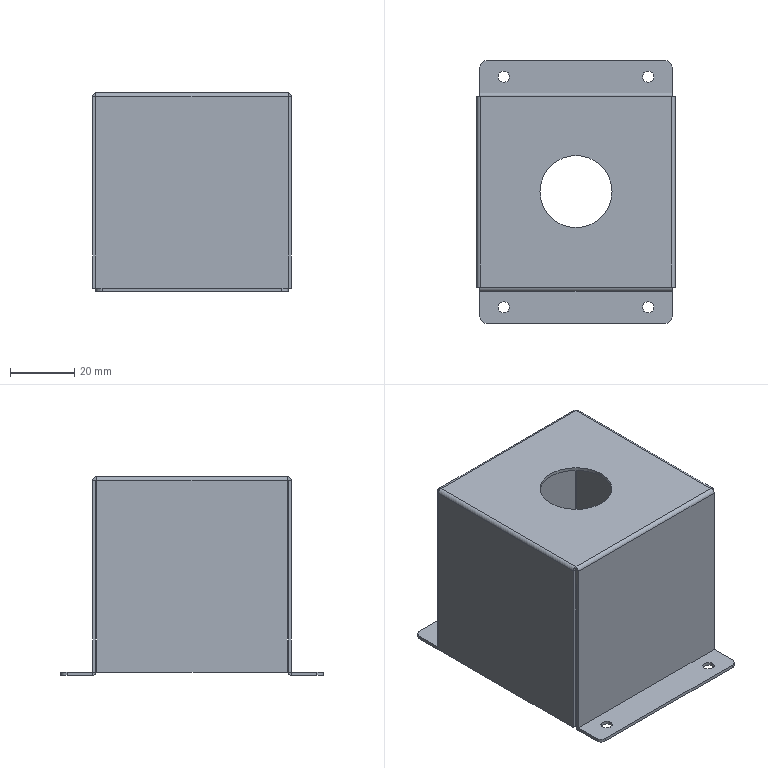Part | SolidWorks | features EdgeFlange 3, Cut 2, Fillet 1, FlatPattern 1, MirrorPattern 1, SMBaseFlange 1, SheetMetal 1 | 1 solid | 70 faces | box 62 x 82 x 62 mm | volume 18974 mm3 | plane 46 | cylinder 24 | commonest cylinder face diameters 3.5 x8 0.4 x4 2.4 x4 4 x4 2 x2 22.5 x2